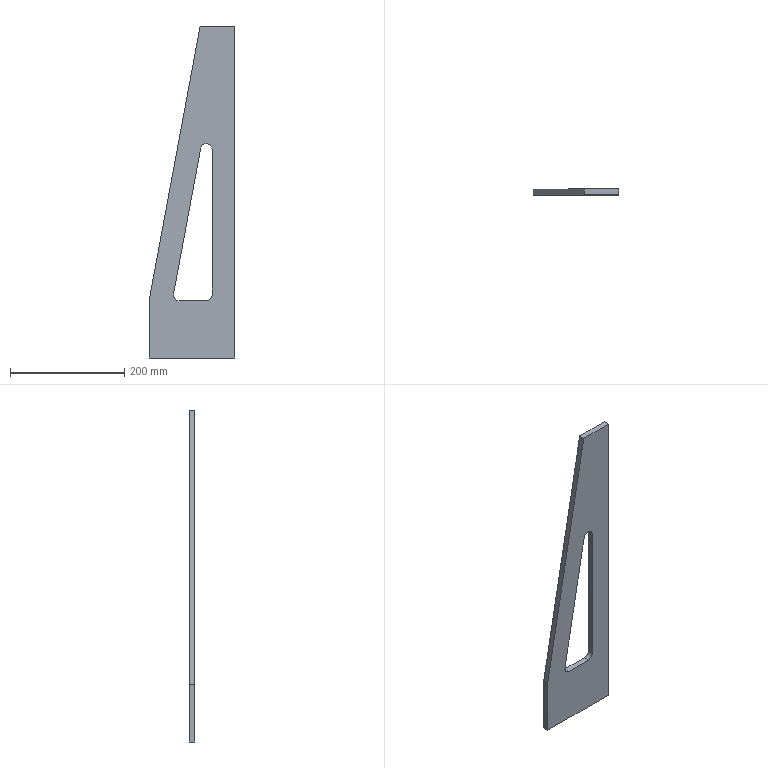Part | SolidWorks | features BaseBody 1 | 1 solid | 14 faces | box 150 x 10 x 580 mm | volume 536622 mm3 | plane 10 | cylinder 4 | commonest cylinder face diameters 20 x4
STEP:
#1=CARTESIAN_POINT('',(-80.,2027.,-925.373));
#2=VERTEX_POINT('',#1);
#3=CARTESIAN_POINT('',(-70.,2027.,-935.373));
#4=VERTEX_POINT('',#3);
#5=CARTESIAN_POINT('',(-80.,2027.,-935.373));
#6=DIRECTION('',(0.,1.,0.));
#7=DIRECTION('',(0.,0.,1.));
#8=AXIS2_PLACEMENT_3D('',#5,#6,#7);
#9=CIRCLE('',#8,10.);
#10=EDGE_CURVE('',#2,#4,#9,.T.);
#11=ORIENTED_EDGE('',*,*,#10,.F.);
#12=CARTESIAN_POINT('',(-80.,2037.,-925.373));
#13=VERTEX_POINT('',#12);
#14=CARTESIAN_POINT('',(-80.,2027.,-925.373));
#15=DIRECTION('',(0.,1.,0.));
#16=VECTOR('',#15,1000.);
#17=LINE('',#14,#16);
#18=EDGE_CURVE('',#2,#13,#17,.T.);
#19=ORIENTED_EDGE('',*,*,#18,.T.);
#20=CARTESIAN_POINT('',(-70.,2037.,-935.373));
#21=VERTEX_POINT('',#20);
#22=CARTESIAN_POINT('',(-80.,2037.,-935.373));
#23=DIRECTION('',(0.,-1.,0.));
#24=DIRECTION('',(0.,0.,1.));
#25=AXIS2_PLACEMENT_3D('',#22,#23,#24);
#26=CIRCLE('',#25,10.);
#27=EDGE_CURVE('',#21,#13,#26,.T.);
#28=ORIENTED_EDGE('',*,*,#27,.F.);
#29=CARTESIAN_POINT('',(-70.,2027.,-935.373));
#30=DIRECTION('',(0.,-1.,0.));
#31=VECTOR('',#30,1000.);
#32=LINE('',#29,#31);
#33=EDGE_CURVE('',#21,#4,#32,.T.);
#34=ORIENTED_EDGE('',*,*,#33,.T.);
#35=EDGE_LOOP('',(#11,#19,#28,#34));
#36=FACE_OUTER_BOUND('',#35,.T.);
#37=CARTESIAN_POINT('',(-80.,2027.,-935.373));
#38=DIRECTION('',(0.,1.,0.));
#39=DIRECTION('',(0.,0.,1.));
#40=AXIS2_PLACEMENT_3D('',#37,#38,#39);
#41=CYLINDRICAL_SURFACE('',#40,10.);
#42=ADVANCED_FACE('',(#36),#41,.F.);
#43=CARTESIAN_POINT('',(-70.,2027.,-1190.));
#44=VERTEX_POINT('',#43);
#45=CARTESIAN_POINT('',(-70.,2027.,-1330.));
#46=DIRECTION('',(0.,0.,-1.));
#47=VECTOR('',#46,1000.);
#48=LINE('',#45,#47);
#49=EDGE_CURVE('',#4,#44,#48,.T.);
#50=ORIENTED_EDGE('',*,*,#49,.T.);
#51=CARTESIAN_POINT('',(-80.,2027.,-1200.));
#52=VERTEX_POINT('',#51);
#53=CARTESIAN_POINT('',(-80.,2027.,-1190.));
#54=DIRECTION('',(0.,1.,0.));
#55=DIRECTION('',(0.,0.,1.));
#56=AXIS2_PLACEMENT_3D('',#53,#54,#55);
#57=CIRCLE('',#56,10.);
#58=EDGE_CURVE('',#44,#52,#57,.T.);
#59=ORIENTED_EDGE('',*,*,#58,.T.);
#60=CARTESIAN_POINT('',(-127.288,2027.,-1200.));
#61=VERTEX_POINT('',#60);
#62=CARTESIAN_POINT('',(-240.,2027.,-1200.));
#63=DIRECTION('',(-1.,0.,0.));
#64=VECTOR('',#63,1000.);
#65=LINE('',#62,#64);
#66=EDGE_CURVE('',#52,#61,#65,.T.);
#67=ORIENTED_EDGE('',*,*,#66,.T.);
#68=CARTESIAN_POINT('',(-137.12,2027.,-1188.174));
#69=VERTEX_POINT('',#68);
#70=CARTESIAN_POINT('',(-127.288,2027.,-1190.));
#71=DIRECTION('',(0.,1.,0.));
#72=DIRECTION('',(0.,0.,1.));
#73=AXIS2_PLACEMENT_3D('',#70,#71,#72);
#74=CIRCLE('',#73,10.);
#75=EDGE_CURVE('',#61,#69,#74,.T.);
#76=ORIENTED_EDGE('',*,*,#75,.T.);
#77=CARTESIAN_POINT('',(-89.832,2027.,-933.547));
#78=VERTEX_POINT('',#77);
#79=CARTESIAN_POINT('',(-137.12,2027.,-1188.174));
#80=DIRECTION('',(0.1826,0.,0.9832));
#81=VECTOR('',#80,1000.);
#82=LINE('',#79,#81);
#83=EDGE_CURVE('',#69,#78,#82,.T.);
#84=ORIENTED_EDGE('',*,*,#83,.T.);
#85=CARTESIAN_POINT('',(-80.,2027.,-935.373));
#86=DIRECTION('',(0.,1.,0.));
#87=DIRECTION('',(0.,0.,1.));
#88=AXIS2_PLACEMENT_3D('',#85,#86,#87);
#89=CIRCLE('',#88,10.);
#90=EDGE_CURVE('',#78,#2,#89,.T.);
#91=ORIENTED_EDGE('',*,*,#90,.T.);
#92=ORIENTED_EDGE('',*,*,#10,.T.);
#93=EDGE_LOOP('',(#50,#59,#67,#76,#84,#91,#92));
#94=FACE_BOUND('',#93,.T.);
#95=CARTESIAN_POINT('',(-30.,2027.,-1300.));
#96=VERTEX_POINT('',#95);
#97=CARTESIAN_POINT('',(-30.,2027.,-720.));
#98=VERTEX_POINT('',#97);
#99=CARTESIAN_POINT('',(-30.,2027.,-1330.));
#100=DIRECTION('',(0.,0.,1.));
#101=VECTOR('',#100,1000.);
#102=LINE('',#99,#101);
#103=EDGE_CURVE('',#96,#98,#102,.T.);
#104=ORIENTED_EDGE('',*,*,#103,.T.);
#105=CARTESIAN_POINT('',(-90.857,2027.,-720.));
#106=VERTEX_POINT('',#105);
#107=CARTESIAN_POINT('',(-240.,2027.,-720.));
#108=DIRECTION('',(-1.,0.,0.));
#109=VECTOR('',#108,1000.);
#110=LINE('',#107,#109);
#111=EDGE_CURVE('',#98,#106,#110,.T.);
#112=ORIENTED_EDGE('',*,*,#111,.T.);
#113=CARTESIAN_POINT('',(-180.,2027.,-1200.));
#114=VERTEX_POINT('',#113);
#115=CARTESIAN_POINT('',(-90.857,2027.,-720.));
#116=DIRECTION('',(-0.1826,0.,-0.9832));
#117=VECTOR('',#116,1000.);
#118=LINE('',#115,#117);
#119=EDGE_CURVE('',#106,#114,#118,.T.);
#120=ORIENTED_EDGE('',*,*,#119,.T.);
#121=CARTESIAN_POINT('',(-180.,2027.,-1300.));
#122=VERTEX_POINT('',#121);
#123=CARTESIAN_POINT('',(-180.,2027.,-1330.));
#124=DIRECTION('',(0.,0.,-1.));
#125=VECTOR('',#124,1000.);
#126=LINE('',#123,#125);
#127=EDGE_CURVE('',#114,#122,#126,.T.);
#128=ORIENTED_EDGE('',*,*,#127,.T.);
#129=CARTESIAN_POINT('',(-240.,2027.,-1300.));
#130=DIRECTION('',(1.,0.,0.));
#131=VECTOR('',#130,1000.);
#132=LINE('',#129,#131);
#133=EDGE_CURVE('',#122,#96,#132,.T.);
#134=ORIENTED_EDGE('',*,*,#133,.T.);
#135=EDGE_LOOP('',(#104,#112,#120,#128,#134));
#136=FACE_OUTER_BOUND('',#135,.T.);
#137=CARTESIAN_POINT('',(-240.,2027.,-1330.));
#138=DIRECTION('',(0.,-1.,0.));
#139=DIRECTION('',(0.,0.,-1.));
#140=AXIS2_PLACEMENT_3D('',#137,#138,#139);
#141=PLANE('',#140);
#142=ADVANCED_FACE('',(#94,#136),#141,.T.);
#143=ORIENTED_EDGE('',*,*,#58,.F.);
#144=CARTESIAN_POINT('',(-70.,2037.,-1190.));
#145=VERTEX_POINT('',#144);
#146=CARTESIAN_POINT('',(-70.,2027.,-1190.));
#147=DIRECTION('',(0.,-1.,0.));
#148=VECTOR('',#147,1000.);
#149=LINE('',#146,#148);
#150=EDGE_CURVE('',#145,#44,#149,.T.);
#151=ORIENTED_EDGE('',*,*,#150,.F.);
#152=CARTESIAN_POINT('',(-80.,2037.,-1200.));
#153=VERTEX_POINT('',#152);
#154=CARTESIAN_POINT('',(-80.,2037.,-1190.));
#155=DIRECTION('',(0.,-1.,0.));
#156=DIRECTION('',(0.,0.,1.));
#157=AXIS2_PLACEMENT_3D('',#154,#155,#156);
#158=CIRCLE('',#157,10.);
#159=EDGE_CURVE('',#153,#145,#158,.T.);
#160=ORIENTED_EDGE('',*,*,#159,.F.);
#161=CARTESIAN_POINT('',(-80.,2027.,-1200.));
#162=DIRECTION('',(0.,1.,0.));
#163=VECTOR('',#162,1000.);
#164=LINE('',#161,#163);
#165=EDGE_CURVE('',#52,#153,#164,.T.);
#166=ORIENTED_EDGE('',*,*,#165,.F.);
#167=EDGE_LOOP('',(#143,#151,#160,#166));
#168=FACE_OUTER_BOUND('',#167,.T.);
#169=CARTESIAN_POINT('',(-80.,2027.,-1190.));
#170=DIRECTION('',(0.,1.,0.));
#171=DIRECTION('',(0.,0.,1.));
#172=AXIS2_PLACEMENT_3D('',#169,#170,#171);
#173=CYLINDRICAL_SURFACE('',#172,10.);
#174=ADVANCED_FACE('',(#168),#173,.F.);
#175=ORIENTED_EDGE('',*,*,#49,.F.);
#176=ORIENTED_EDGE('',*,*,#33,.F.);
#177=CARTESIAN_POINT('',(-70.,2037.,-935.373));
#178=DIRECTION('',(0.,0.,1.));
#179=VECTOR('',#178,1000.);
#180=LINE('',#177,#179);
#181=EDGE_CURVE('',#145,#21,#180,.T.);
#182=ORIENTED_EDGE('',*,*,#181,.F.);
#183=ORIENTED_EDGE('',*,*,#150,.T.);
#184=EDGE_LOOP('',(#175,#176,#182,#183));
#185=FACE_OUTER_BOUND('',#184,.T.);
#186=CARTESIAN_POINT('',(-70.,2027.,-935.373));
#187=DIRECTION('',(1.,0.,0.));
#188=DIRECTION('',(0.,0.,-1.));
#189=AXIS2_PLACEMENT_3D('',#186,#187,#188);
#190=PLANE('',#189);
#191=ADVANCED_FACE('',(#185),#190,.F.);
#192=ORIENTED_EDGE('',*,*,#18,.F.);
#193=ORIENTED_EDGE('',*,*,#90,.F.);
#194=CARTESIAN_POINT('',(-89.832,2037.,-933.547));
#195=VERTEX_POINT('',#194);
#196=CARTESIAN_POINT('',(-89.832,2027.,-933.547));
#197=DIRECTION('',(0.,-1.,0.));
#198=VECTOR('',#197,1000.);
#199=LINE('',#196,#198);
#200=EDGE_CURVE('',#195,#78,#199,.T.);
#201=ORIENTED_EDGE('',*,*,#200,.F.);
#202=CARTESIAN_POINT('',(-80.,2037.,-935.373));
#203=DIRECTION('',(0.,-1.,0.));
#204=DIRECTION('',(0.,0.,1.));
#205=AXIS2_PLACEMENT_3D('',#202,#203,#204);
#206=CIRCLE('',#205,10.);
#207=EDGE_CURVE('',#13,#195,#206,.T.);
#208=ORIENTED_EDGE('',*,*,#207,.F.);
#209=EDGE_LOOP('',(#192,#193,#201,#208));
#210=FACE_OUTER_BOUND('',#209,.T.);
#211=CARTESIAN_POINT('',(-80.,2027.,-935.373));
#212=DIRECTION('',(0.,1.,0.));
#213=DIRECTION('',(0.,0.,1.));
#214=AXIS2_PLACEMENT_3D('',#211,#212,#213);
#215=CYLINDRICAL_SURFACE('',#214,10.);
#216=ADVANCED_FACE('',(#210),#215,.F.);
#217=ORIENTED_EDGE('',*,*,#83,.F.);
#218=CARTESIAN_POINT('',(-137.12,2037.,-1188.174));
#219=VERTEX_POINT('',#218);
#220=CARTESIAN_POINT('',(-137.12,2027.,-1188.174));
#221=DIRECTION('',(0.,-1.,0.));
#222=VECTOR('',#221,1000.);
#223=LINE('',#220,#222);
#224=EDGE_CURVE('',#219,#69,#223,.T.);
#225=ORIENTED_EDGE('',*,*,#224,.F.);
#226=CARTESIAN_POINT('',(-137.12,2037.,-1188.174));
#227=DIRECTION('',(-0.1826,0.,-0.9832));
#228=VECTOR('',#227,1000.);
#229=LINE('',#226,#228);
#230=EDGE_CURVE('',#195,#219,#229,.T.);
#231=ORIENTED_EDGE('',*,*,#230,.F.);
#232=ORIENTED_EDGE('',*,*,#200,.T.);
#233=EDGE_LOOP('',(#217,#225,#231,#232));
#234=FACE_OUTER_BOUND('',#233,.T.);
#235=CARTESIAN_POINT('',(-137.12,2027.,-1188.174));
#236=DIRECTION('',(-0.9832,0.,0.1826));
#237=DIRECTION('',(0.1826,0.,0.9832));
#238=AXIS2_PLACEMENT_3D('',#235,#236,#237);
#239=PLANE('',#238);
#240=ADVANCED_FACE('',(#234),#239,.F.);
#241=ORIENTED_EDGE('',*,*,#224,.T.);
#242=ORIENTED_EDGE('',*,*,#75,.F.);
#243=CARTESIAN_POINT('',(-127.288,2037.,-1200.));
#244=VERTEX_POINT('',#243);
#245=CARTESIAN_POINT('',(-127.288,2027.,-1200.));
#246=DIRECTION('',(0.,-1.,0.));
#247=VECTOR('',#246,1000.);
#248=LINE('',#245,#247);
#249=EDGE_CURVE('',#244,#61,#248,.T.);
#250=ORIENTED_EDGE('',*,*,#249,.F.);
#251=CARTESIAN_POINT('',(-127.288,2037.,-1190.));
#252=DIRECTION('',(0.,-1.,0.));
#253=DIRECTION('',(0.,0.,1.));
#254=AXIS2_PLACEMENT_3D('',#251,#252,#253);
#255=CIRCLE('',#254,10.);
#256=EDGE_CURVE('',#219,#244,#255,.T.);
#257=ORIENTED_EDGE('',*,*,#256,.F.);
#258=EDGE_LOOP('',(#241,#242,#250,#257));
#259=FACE_OUTER_BOUND('',#258,.T.);
#260=CARTESIAN_POINT('',(-127.288,2027.,-1190.));
#261=DIRECTION('',(0.,1.,0.));
#262=DIRECTION('',(0.,0.,1.));
#263=AXIS2_PLACEMENT_3D('',#260,#261,#262);
#264=CYLINDRICAL_SURFACE('',#263,10.);
#265=ADVANCED_FACE('',(#259),#264,.F.);
#266=ORIENTED_EDGE('',*,*,#66,.F.);
#267=ORIENTED_EDGE('',*,*,#165,.T.);
#268=CARTESIAN_POINT('',(-80.,2037.,-1200.));
#269=DIRECTION('',(1.,0.,0.));
#270=VECTOR('',#269,1000.);
#271=LINE('',#268,#270);
#272=EDGE_CURVE('',#244,#153,#271,.T.);
#273=ORIENTED_EDGE('',*,*,#272,.F.);
#274=ORIENTED_EDGE('',*,*,#249,.T.);
#275=EDGE_LOOP('',(#266,#267,#273,#274));
#276=FACE_OUTER_BOUND('',#275,.T.);
#277=CARTESIAN_POINT('',(-80.,2027.,-1200.));
#278=DIRECTION('',(0.,0.,-1.));
#279=DIRECTION('',(-1.,0.,0.));
#280=AXIS2_PLACEMENT_3D('',#277,#278,#279);
#281=PLANE('',#280);
#282=ADVANCED_FACE('',(#276),#281,.F.);
#283=CARTESIAN_POINT('',(-90.857,2037.,-720.));
#284=VERTEX_POINT('',#283);
#285=CARTESIAN_POINT('',(-30.,2037.,-720.));
#286=VERTEX_POINT('',#285);
#287=CARTESIAN_POINT('',(-240.,2037.,-720.));
#288=DIRECTION('',(1.,0.,0.));
#289=VECTOR('',#288,1000.);
#290=LINE('',#287,#289);
#291=EDGE_CURVE('',#284,#286,#290,.T.);
#292=ORIENTED_EDGE('',*,*,#291,.F.);
#293=CARTESIAN_POINT('',(-90.857,2402.,-720.));
#294=DIRECTION('',(0.,1.,0.));
#295=VECTOR('',#294,1000.);
#296=LINE('',#293,#295);
#297=EDGE_CURVE('',#106,#284,#296,.T.);
#298=ORIENTED_EDGE('',*,*,#297,.F.);
#299=ORIENTED_EDGE('',*,*,#111,.F.);
#300=CARTESIAN_POINT('',(-30.,2402.,-720.));
#301=DIRECTION('',(0.,-1.,0.));
#302=VECTOR('',#301,1000.);
#303=LINE('',#300,#302);
#304=EDGE_CURVE('',#286,#98,#303,.T.);
#305=ORIENTED_EDGE('',*,*,#304,.F.);
#306=EDGE_LOOP('',(#292,#298,#299,#305));
#307=FACE_OUTER_BOUND('',#306,.T.);
#308=CARTESIAN_POINT('',(-240.,2402.,-720.));
#309=DIRECTION('',(0.,0.,-1.));
#310=DIRECTION('',(-1.,0.,0.));
#311=AXIS2_PLACEMENT_3D('',#308,#309,#310);
#312=PLANE('',#311);
#313=ADVANCED_FACE('',(#307),#312,.F.);
#314=CARTESIAN_POINT('',(-30.,2037.,-1300.));
#315=VERTEX_POINT('',#314);
#316=CARTESIAN_POINT('',(-30.,2037.,-1300.));
#317=DIRECTION('',(0.,0.,1.));
#318=VECTOR('',#317,1000.);
#319=LINE('',#316,#318);
#320=EDGE_CURVE('',#315,#286,#319,.T.);
#321=ORIENTED_EDGE('',*,*,#320,.T.);
#322=ORIENTED_EDGE('',*,*,#304,.T.);
#323=ORIENTED_EDGE('',*,*,#103,.F.);
#324=CARTESIAN_POINT('',(-30.,2027.,-1300.));
#325=DIRECTION('',(0.,1.,0.));
#326=VECTOR('',#325,1000.);
#327=LINE('',#324,#326);
#328=EDGE_CURVE('',#96,#315,#327,.T.);
#329=ORIENTED_EDGE('',*,*,#328,.T.);
#330=EDGE_LOOP('',(#321,#322,#323,#329));
#331=FACE_OUTER_BOUND('',#330,.T.);
#332=CARTESIAN_POINT('',(-30.,2027.,-1300.));
#333=DIRECTION('',(1.,0.,0.));
#334=DIRECTION('',(0.,0.,-1.));
#335=AXIS2_PLACEMENT_3D('',#332,#333,#334);
#336=PLANE('',#335);
#337=ADVANCED_FACE('',(#331),#336,.T.);
#338=CARTESIAN_POINT('',(-180.,2037.,-1300.));
#339=VERTEX_POINT('',#338);
#340=CARTESIAN_POINT('',(-180.,2027.,-1300.));
#341=DIRECTION('',(0.,1.,0.));
#342=VECTOR('',#341,1000.);
#343=LINE('',#340,#342);
#344=EDGE_CURVE('',#122,#339,#343,.T.);
#345=ORIENTED_EDGE('',*,*,#344,.T.);
#346=CARTESIAN_POINT('',(-180.,2037.,-1300.));
#347=DIRECTION('',(1.,0.,0.));
#348=VECTOR('',#347,1000.);
#349=LINE('',#346,#348);
#350=EDGE_CURVE('',#339,#315,#349,.T.);
#351=ORIENTED_EDGE('',*,*,#350,.T.);
#352=ORIENTED_EDGE('',*,*,#328,.F.);
#353=ORIENTED_EDGE('',*,*,#133,.F.);
#354=EDGE_LOOP('',(#345,#351,#352,#353));
#355=FACE_OUTER_BOUND('',#354,.T.);
#356=CARTESIAN_POINT('',(-180.,2027.,-1300.));
#357=DIRECTION('',(0.,0.,-1.));
#358=DIRECTION('',(-1.,0.,0.));
#359=AXIS2_PLACEMENT_3D('',#356,#357,#358);
#360=PLANE('',#359);
#361=ADVANCED_FACE('',(#355),#360,.T.);
#362=CARTESIAN_POINT('',(-180.,2037.,-1200.));
#363=VERTEX_POINT('',#362);
#364=CARTESIAN_POINT('',(-180.,2027.,-1200.));
#365=DIRECTION('',(0.,1.,0.));
#366=VECTOR('',#365,1000.);
#367=LINE('',#364,#366);
#368=EDGE_CURVE('',#114,#363,#367,.T.);
#369=ORIENTED_EDGE('',*,*,#368,.T.);
#370=CARTESIAN_POINT('',(-180.,2037.,-1200.));
#371=DIRECTION('',(0.,0.,-1.));
#372=VECTOR('',#371,1000.);
#373=LINE('',#370,#372);
#374=EDGE_CURVE('',#363,#339,#373,.T.);
#375=ORIENTED_EDGE('',*,*,#374,.T.);
#376=ORIENTED_EDGE('',*,*,#344,.F.);
#377=ORIENTED_EDGE('',*,*,#127,.F.);
#378=EDGE_LOOP('',(#369,#375,#376,#377));
#379=FACE_OUTER_BOUND('',#378,.T.);
#380=CARTESIAN_POINT('',(-180.,2027.,-1200.));
#381=DIRECTION('',(-1.,0.,0.));
#382=DIRECTION('',(0.,0.,1.));
#383=AXIS2_PLACEMENT_3D('',#380,#381,#382);
#384=PLANE('',#383);
#385=ADVANCED_FACE('',(#379),#384,.T.);
#386=ORIENTED_EDGE('',*,*,#119,.F.);
#387=ORIENTED_EDGE('',*,*,#297,.T.);
#388=CARTESIAN_POINT('',(-50.,2037.,-500.));
#389=DIRECTION('',(-0.1826,0.,-0.9832));
#390=VECTOR('',#389,1000.);
#391=LINE('',#388,#390);
#392=EDGE_CURVE('',#284,#363,#391,.T.);
#393=ORIENTED_EDGE('',*,*,#392,.T.);
#394=ORIENTED_EDGE('',*,*,#368,.F.);
#395=EDGE_LOOP('',(#386,#387,#393,#394));
#396=FACE_OUTER_BOUND('',#395,.T.);
#397=CARTESIAN_POINT('',(-50.,2027.,-500.));
#398=DIRECTION('',(-0.9832,0.,0.1826));
#399=DIRECTION('',(0.1826,0.,0.9832));
#400=AXIS2_PLACEMENT_3D('',#397,#398,#399);
#401=PLANE('',#400);
#402=ADVANCED_FACE('',(#396),#401,.T.);
#403=ORIENTED_EDGE('',*,*,#181,.T.);
#404=ORIENTED_EDGE('',*,*,#27,.T.);
#405=ORIENTED_EDGE('',*,*,#207,.T.);
#406=ORIENTED_EDGE('',*,*,#230,.T.);
#407=ORIENTED_EDGE('',*,*,#256,.T.);
#408=ORIENTED_EDGE('',*,*,#272,.T.);
#409=ORIENTED_EDGE('',*,*,#159,.T.);
#410=EDGE_LOOP('',(#403,#404,#405,#406,#407,#408,#409));
#411=FACE_BOUND('',#410,.T.);
#412=ORIENTED_EDGE('',*,*,#320,.F.);
#413=ORIENTED_EDGE('',*,*,#350,.F.);
#414=ORIENTED_EDGE('',*,*,#374,.F.);
#415=ORIENTED_EDGE('',*,*,#392,.F.);
#416=ORIENTED_EDGE('',*,*,#291,.T.);
#417=EDGE_LOOP('',(#412,#413,#414,#415,#416));
#418=FACE_OUTER_BOUND('',#417,.T.);
#419=CARTESIAN_POINT('',(-240.,2037.,-1330.));
#420=DIRECTION('',(0.,-1.,0.));
#421=DIRECTION('',(0.,0.,-1.));
#422=AXIS2_PLACEMENT_3D('',#419,#420,#421);
#423=PLANE('',#422);
#424=ADVANCED_FACE('',(#411,#418),#423,.F.);
#425=CLOSED_SHELL('',(#42,#142,#174,#191,#216,#240,#265,#282,#313,#337,#361,#385,#402,#424));
#426=MANIFOLD_SOLID_BREP('',#425);
#427=CARTESIAN_POINT('',(0.,0.,0.));
#428=DIRECTION('',(0.,0.,1.));
#429=DIRECTION('',(1.,0.,0.));
#430=AXIS2_PLACEMENT_3D('',#427,#428,#429);
#431=(LENGTH_UNIT()NAMED_UNIT(*)SI_UNIT(.MILLI.,.METRE.));
#432=UNCERTAINTY_MEASURE_WITH_UNIT(LENGTH_MEASURE(0.00001),#431,'','');
#433=(NAMED_UNIT(*)PLANE_ANGLE_UNIT()SI_UNIT($,.RADIAN.));
#434=(NAMED_UNIT(*)SI_UNIT($,.STERADIAN.)SOLID_ANGLE_UNIT());
#435=(GEOMETRIC_REPRESENTATION_CONTEXT(3)GLOBAL_UNCERTAINTY_ASSIGNED_CONTEXT((#432))GLOBAL_UNIT_ASSIGNED_CONTEXT((#431,#433,#434))REPRESENTATION_CONTEXT('',''));
#436=ADVANCED_BREP_SHAPE_REPRESENTATION('',(#426,#430),#435);